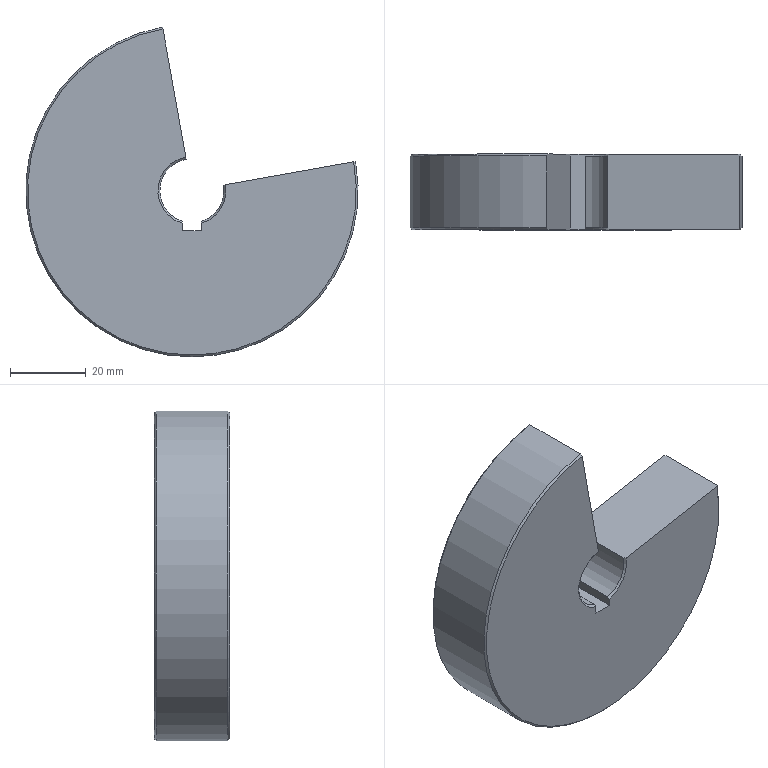Part | STEP file | Cuon T phu H01_6 | 1 solid | 18 faces | box 88 x 20 x 87.312 mm | volume 87542 mm3 | cone 7 | plane 7 | cylinder 4 | commonest cylinder face diameters 17 x2 88 x2